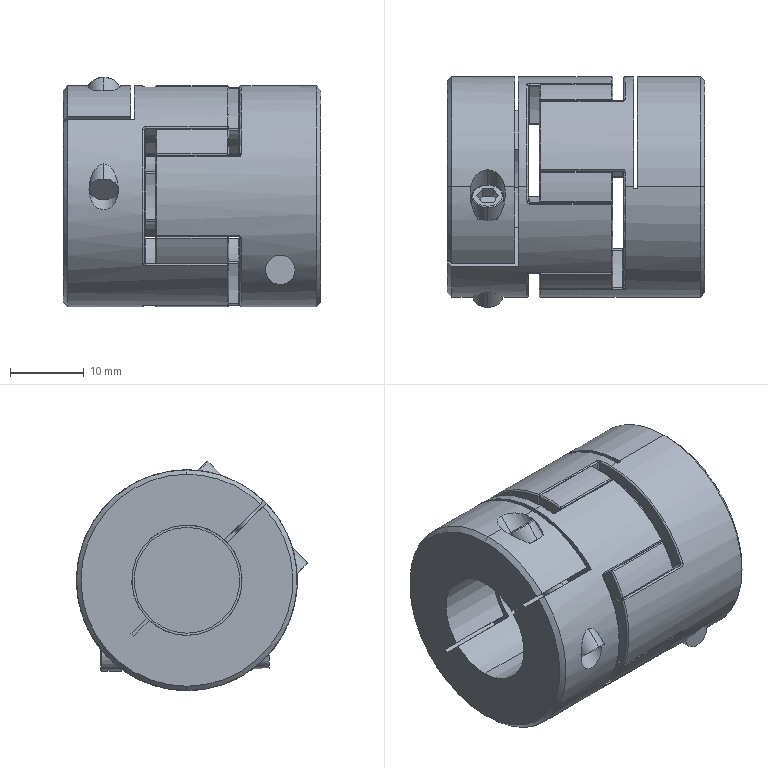Part | SolidWorks | features ICE 26, Fillet 5, CirPattern 4, Chamfer 2, Extrusion 2, Revolution 2 | 3 solids | 406 faces | box 35 x 31.385 x 31.157 mm | volume 18507 mm3 | torus 146 | cylinder 135 | sphere 58 | plane 50 | spline 12 | cone 5 | commonest cylinder face diameters 0.4 x58 18 x36 30 x13 4 x10 14.4 x4 15 x4